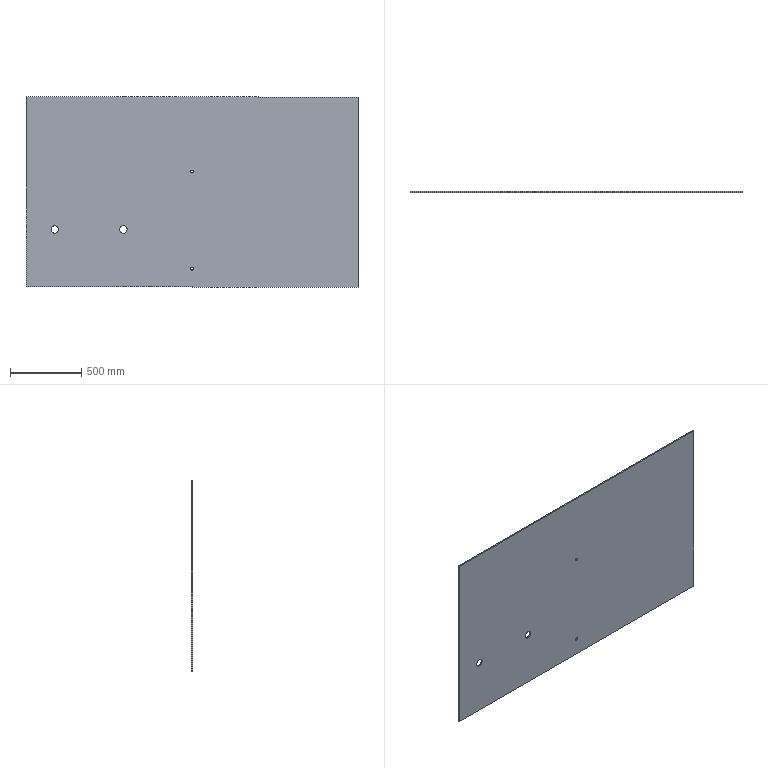Part | SolidWorks | features Extrusion 1 | 1 solid | 14 faces | box 2324 x 8 x 1330 mm | volume 24688354 mm3 | cylinder 8 | plane 6 | commonest cylinder face diameters 20 x4 52 x4
STEP:
#1=CARTESIAN_POINT('',(-960.,4.,-288.));
#2=VERTEX_POINT('',#1);
#3=CARTESIAN_POINT('',(-960.,4.,-236.));
#4=VERTEX_POINT('',#3);
#5=CARTESIAN_POINT('',(-960.,4.,-262.));
#6=DIRECTION('',(0.,1.,0.));
#7=DIRECTION('',(0.,0.,1.));
#8=AXIS2_PLACEMENT_3D('',#5,#6,#7);
#9=CIRCLE('',#8,26.);
#10=EDGE_CURVE('',#2,#4,#9,.T.);
#11=ORIENTED_EDGE('',*,*,#10,.T.);
#12=CARTESIAN_POINT('',(-960.,-4.,-236.));
#13=VERTEX_POINT('',#12);
#14=CARTESIAN_POINT('',(-960.,4.,-236.));
#15=DIRECTION('',(0.,-1.,0.));
#16=VECTOR('',#15,1000.);
#17=LINE('',#14,#16);
#18=EDGE_CURVE('',#4,#13,#17,.T.);
#19=ORIENTED_EDGE('',*,*,#18,.T.);
#20=CARTESIAN_POINT('',(-960.,-4.,-288.));
#21=VERTEX_POINT('',#20);
#22=CARTESIAN_POINT('',(-960.,-4.,-262.));
#23=DIRECTION('',(0.,1.,0.));
#24=DIRECTION('',(0.,0.,1.));
#25=AXIS2_PLACEMENT_3D('',#22,#23,#24);
#26=CIRCLE('',#25,26.);
#27=EDGE_CURVE('',#21,#13,#26,.T.);
#28=ORIENTED_EDGE('',*,*,#27,.F.);
#29=CARTESIAN_POINT('',(-960.,4.,-288.));
#30=DIRECTION('',(0.,-1.,0.));
#31=VECTOR('',#30,1000.);
#32=LINE('',#29,#31);
#33=EDGE_CURVE('',#2,#21,#32,.T.);
#34=ORIENTED_EDGE('',*,*,#33,.F.);
#35=EDGE_LOOP('',(#11,#19,#28,#34));
#36=FACE_OUTER_BOUND('',#35,.T.);
#37=CARTESIAN_POINT('',(-960.,4.,-262.));
#38=DIRECTION('',(0.,-1.,0.));
#39=DIRECTION('',(0.,0.,-1.));
#40=AXIS2_PLACEMENT_3D('',#37,#38,#39);
#41=CYLINDRICAL_SURFACE('',#40,26.);
#42=ADVANCED_FACE('',(#36),#41,.F.);
#43=CARTESIAN_POINT('',(-480.,4.,-288.));
#44=VERTEX_POINT('',#43);
#45=CARTESIAN_POINT('',(-480.,4.,-236.));
#46=VERTEX_POINT('',#45);
#47=CARTESIAN_POINT('',(-480.,4.,-262.));
#48=DIRECTION('',(0.,1.,0.));
#49=DIRECTION('',(0.,0.,1.));
#50=AXIS2_PLACEMENT_3D('',#47,#48,#49);
#51=CIRCLE('',#50,26.);
#52=EDGE_CURVE('',#44,#46,#51,.T.);
#53=ORIENTED_EDGE('',*,*,#52,.T.);
#54=CARTESIAN_POINT('',(-480.,-4.,-236.));
#55=VERTEX_POINT('',#54);
#56=CARTESIAN_POINT('',(-480.,4.,-236.));
#57=DIRECTION('',(0.,-1.,0.));
#58=VECTOR('',#57,1000.);
#59=LINE('',#56,#58);
#60=EDGE_CURVE('',#46,#55,#59,.T.);
#61=ORIENTED_EDGE('',*,*,#60,.T.);
#62=CARTESIAN_POINT('',(-480.,-4.,-288.));
#63=VERTEX_POINT('',#62);
#64=CARTESIAN_POINT('',(-480.,-4.,-262.));
#65=DIRECTION('',(0.,1.,0.));
#66=DIRECTION('',(0.,0.,1.));
#67=AXIS2_PLACEMENT_3D('',#64,#65,#66);
#68=CIRCLE('',#67,26.);
#69=EDGE_CURVE('',#63,#55,#68,.T.);
#70=ORIENTED_EDGE('',*,*,#69,.F.);
#71=CARTESIAN_POINT('',(-480.,4.,-288.));
#72=DIRECTION('',(0.,-1.,0.));
#73=VECTOR('',#72,1000.);
#74=LINE('',#71,#73);
#75=EDGE_CURVE('',#44,#63,#74,.T.);
#76=ORIENTED_EDGE('',*,*,#75,.F.);
#77=EDGE_LOOP('',(#53,#61,#70,#76));
#78=FACE_OUTER_BOUND('',#77,.T.);
#79=CARTESIAN_POINT('',(-480.,4.,-262.));
#80=DIRECTION('',(0.,-1.,0.));
#81=DIRECTION('',(0.,0.,-1.));
#82=AXIS2_PLACEMENT_3D('',#79,#80,#81);
#83=CYLINDRICAL_SURFACE('',#82,26.);
#84=ADVANCED_FACE('',(#78),#83,.F.);
#85=CARTESIAN_POINT('',(0.,4.,133.));
#86=VERTEX_POINT('',#85);
#87=CARTESIAN_POINT('',(0.,4.,153.));
#88=VERTEX_POINT('',#87);
#89=CARTESIAN_POINT('',(0.,4.,143.));
#90=DIRECTION('',(0.,1.,0.));
#91=DIRECTION('',(0.,0.,1.));
#92=AXIS2_PLACEMENT_3D('',#89,#90,#91);
#93=CIRCLE('',#92,10.);
#94=EDGE_CURVE('',#86,#88,#93,.T.);
#95=ORIENTED_EDGE('',*,*,#94,.T.);
#96=CARTESIAN_POINT('',(0.,-4.,153.));
#97=VERTEX_POINT('',#96);
#98=CARTESIAN_POINT('',(0.,4.,153.));
#99=DIRECTION('',(0.,-1.,0.));
#100=VECTOR('',#99,1000.);
#101=LINE('',#98,#100);
#102=EDGE_CURVE('',#88,#97,#101,.T.);
#103=ORIENTED_EDGE('',*,*,#102,.T.);
#104=CARTESIAN_POINT('',(0.,-4.,133.));
#105=VERTEX_POINT('',#104);
#106=CARTESIAN_POINT('',(0.,-4.,143.));
#107=DIRECTION('',(0.,1.,0.));
#108=DIRECTION('',(0.,0.,1.));
#109=AXIS2_PLACEMENT_3D('',#106,#107,#108);
#110=CIRCLE('',#109,10.);
#111=EDGE_CURVE('',#105,#97,#110,.T.);
#112=ORIENTED_EDGE('',*,*,#111,.F.);
#113=CARTESIAN_POINT('',(0.,4.,133.));
#114=DIRECTION('',(0.,-1.,0.));
#115=VECTOR('',#114,1000.);
#116=LINE('',#113,#115);
#117=EDGE_CURVE('',#86,#105,#116,.T.);
#118=ORIENTED_EDGE('',*,*,#117,.F.);
#119=EDGE_LOOP('',(#95,#103,#112,#118));
#120=FACE_OUTER_BOUND('',#119,.T.);
#121=CARTESIAN_POINT('',(0.,4.,143.));
#122=DIRECTION('',(0.,-1.,0.));
#123=DIRECTION('',(0.,0.,-1.));
#124=AXIS2_PLACEMENT_3D('',#121,#122,#123);
#125=CYLINDRICAL_SURFACE('',#124,10.);
#126=ADVANCED_FACE('',(#120),#125,.F.);
#127=CARTESIAN_POINT('',(0.,4.,-547.));
#128=VERTEX_POINT('',#127);
#129=CARTESIAN_POINT('',(0.,4.,-527.));
#130=VERTEX_POINT('',#129);
#131=CARTESIAN_POINT('',(0.,4.,-537.));
#132=DIRECTION('',(0.,1.,0.));
#133=DIRECTION('',(0.,0.,1.));
#134=AXIS2_PLACEMENT_3D('',#131,#132,#133);
#135=CIRCLE('',#134,10.);
#136=EDGE_CURVE('',#128,#130,#135,.T.);
#137=ORIENTED_EDGE('',*,*,#136,.T.);
#138=CARTESIAN_POINT('',(0.,-4.,-527.));
#139=VERTEX_POINT('',#138);
#140=CARTESIAN_POINT('',(0.,4.,-527.));
#141=DIRECTION('',(0.,-1.,0.));
#142=VECTOR('',#141,1000.);
#143=LINE('',#140,#142);
#144=EDGE_CURVE('',#130,#139,#143,.T.);
#145=ORIENTED_EDGE('',*,*,#144,.T.);
#146=CARTESIAN_POINT('',(0.,-4.,-547.));
#147=VERTEX_POINT('',#146);
#148=CARTESIAN_POINT('',(0.,-4.,-537.));
#149=DIRECTION('',(0.,1.,0.));
#150=DIRECTION('',(0.,0.,1.));
#151=AXIS2_PLACEMENT_3D('',#148,#149,#150);
#152=CIRCLE('',#151,10.);
#153=EDGE_CURVE('',#147,#139,#152,.T.);
#154=ORIENTED_EDGE('',*,*,#153,.F.);
#155=CARTESIAN_POINT('',(0.,4.,-547.));
#156=DIRECTION('',(0.,-1.,0.));
#157=VECTOR('',#156,1000.);
#158=LINE('',#155,#157);
#159=EDGE_CURVE('',#128,#147,#158,.T.);
#160=ORIENTED_EDGE('',*,*,#159,.F.);
#161=EDGE_LOOP('',(#137,#145,#154,#160));
#162=FACE_OUTER_BOUND('',#161,.T.);
#163=CARTESIAN_POINT('',(0.,4.,-537.));
#164=DIRECTION('',(0.,-1.,0.));
#165=DIRECTION('',(0.,0.,-1.));
#166=AXIS2_PLACEMENT_3D('',#163,#164,#165);
#167=CYLINDRICAL_SURFACE('',#166,10.);
#168=ADVANCED_FACE('',(#162),#167,.F.);
#169=CARTESIAN_POINT('',(1162.,4.,665.));
#170=VERTEX_POINT('',#169);
#171=CARTESIAN_POINT('',(1162.,4.,-665.));
#172=VERTEX_POINT('',#171);
#173=CARTESIAN_POINT('',(1162.,4.,665.));
#174=DIRECTION('',(0.,0.,-1.));
#175=VECTOR('',#174,1000.);
#176=LINE('',#173,#175);
#177=EDGE_CURVE('',#170,#172,#176,.T.);
#178=ORIENTED_EDGE('',*,*,#177,.T.);
#179=CARTESIAN_POINT('',(-1162.,4.,-665.));
#180=VERTEX_POINT('',#179);
#181=CARTESIAN_POINT('',(-1162.,4.,-665.));
#182=DIRECTION('',(-1.,0.,0.));
#183=VECTOR('',#182,1000.);
#184=LINE('',#181,#183);
#185=EDGE_CURVE('',#172,#180,#184,.T.);
#186=ORIENTED_EDGE('',*,*,#185,.T.);
#187=CARTESIAN_POINT('',(-1162.,4.,665.));
#188=VERTEX_POINT('',#187);
#189=CARTESIAN_POINT('',(-1162.,4.,665.));
#190=DIRECTION('',(0.,0.,1.));
#191=VECTOR('',#190,1000.);
#192=LINE('',#189,#191);
#193=EDGE_CURVE('',#180,#188,#192,.T.);
#194=ORIENTED_EDGE('',*,*,#193,.T.);
#195=CARTESIAN_POINT('',(-1162.,4.,665.));
#196=DIRECTION('',(1.,0.,0.));
#197=VECTOR('',#196,1000.);
#198=LINE('',#195,#197);
#199=EDGE_CURVE('',#188,#170,#198,.T.);
#200=ORIENTED_EDGE('',*,*,#199,.T.);
#201=EDGE_LOOP('',(#178,#186,#194,#200));
#202=FACE_OUTER_BOUND('',#201,.T.);
#203=ORIENTED_EDGE('',*,*,#136,.F.);
#204=CARTESIAN_POINT('',(0.,4.,-537.));
#205=DIRECTION('',(0.,1.,0.));
#206=DIRECTION('',(0.,0.,1.));
#207=AXIS2_PLACEMENT_3D('',#204,#205,#206);
#208=CIRCLE('',#207,10.);
#209=EDGE_CURVE('',#130,#128,#208,.T.);
#210=ORIENTED_EDGE('',*,*,#209,.F.);
#211=EDGE_LOOP('',(#203,#210));
#212=FACE_BOUND('',#211,.T.);
#213=ORIENTED_EDGE('',*,*,#94,.F.);
#214=CARTESIAN_POINT('',(0.,4.,143.));
#215=DIRECTION('',(0.,1.,0.));
#216=DIRECTION('',(0.,0.,1.));
#217=AXIS2_PLACEMENT_3D('',#214,#215,#216);
#218=CIRCLE('',#217,10.);
#219=EDGE_CURVE('',#88,#86,#218,.T.);
#220=ORIENTED_EDGE('',*,*,#219,.F.);
#221=EDGE_LOOP('',(#213,#220));
#222=FACE_BOUND('',#221,.T.);
#223=ORIENTED_EDGE('',*,*,#52,.F.);
#224=CARTESIAN_POINT('',(-480.,4.,-262.));
#225=DIRECTION('',(0.,1.,0.));
#226=DIRECTION('',(0.,0.,1.));
#227=AXIS2_PLACEMENT_3D('',#224,#225,#226);
#228=CIRCLE('',#227,26.);
#229=EDGE_CURVE('',#46,#44,#228,.T.);
#230=ORIENTED_EDGE('',*,*,#229,.F.);
#231=EDGE_LOOP('',(#223,#230));
#232=FACE_BOUND('',#231,.T.);
#233=ORIENTED_EDGE('',*,*,#10,.F.);
#234=CARTESIAN_POINT('',(-960.,4.,-262.));
#235=DIRECTION('',(0.,1.,0.));
#236=DIRECTION('',(0.,0.,1.));
#237=AXIS2_PLACEMENT_3D('',#234,#235,#236);
#238=CIRCLE('',#237,26.);
#239=EDGE_CURVE('',#4,#2,#238,.T.);
#240=ORIENTED_EDGE('',*,*,#239,.F.);
#241=EDGE_LOOP('',(#233,#240));
#242=FACE_BOUND('',#241,.T.);
#243=CARTESIAN_POINT('',(0.,4.,0.));
#244=DIRECTION('',(0.,-1.,0.));
#245=DIRECTION('',(0.,0.,-1.));
#246=AXIS2_PLACEMENT_3D('',#243,#244,#245);
#247=PLANE('',#246);
#248=ADVANCED_FACE('',(#202,#212,#222,#232,#242),#247,.F.);
#249=ORIENTED_EDGE('',*,*,#69,.T.);
#250=CARTESIAN_POINT('',(-480.,-4.,-262.));
#251=DIRECTION('',(0.,1.,0.));
#252=DIRECTION('',(0.,0.,1.));
#253=AXIS2_PLACEMENT_3D('',#250,#251,#252);
#254=CIRCLE('',#253,26.);
#255=EDGE_CURVE('',#55,#63,#254,.T.);
#256=ORIENTED_EDGE('',*,*,#255,.T.);
#257=EDGE_LOOP('',(#249,#256));
#258=FACE_BOUND('',#257,.T.);
#259=ORIENTED_EDGE('',*,*,#153,.T.);
#260=CARTESIAN_POINT('',(0.,-4.,-537.));
#261=DIRECTION('',(0.,1.,0.));
#262=DIRECTION('',(0.,0.,1.));
#263=AXIS2_PLACEMENT_3D('',#260,#261,#262);
#264=CIRCLE('',#263,10.);
#265=EDGE_CURVE('',#139,#147,#264,.T.);
#266=ORIENTED_EDGE('',*,*,#265,.T.);
#267=EDGE_LOOP('',(#259,#266));
#268=FACE_BOUND('',#267,.T.);
#269=CARTESIAN_POINT('',(1162.,-4.,665.));
#270=VERTEX_POINT('',#269);
#271=CARTESIAN_POINT('',(1162.,-4.,-665.));
#272=VERTEX_POINT('',#271);
#273=CARTESIAN_POINT('',(1162.,-4.,665.));
#274=DIRECTION('',(0.,0.,-1.));
#275=VECTOR('',#274,1000.);
#276=LINE('',#273,#275);
#277=EDGE_CURVE('',#270,#272,#276,.T.);
#278=ORIENTED_EDGE('',*,*,#277,.F.);
#279=CARTESIAN_POINT('',(-1162.,-4.,665.));
#280=VERTEX_POINT('',#279);
#281=CARTESIAN_POINT('',(-1162.,-4.,665.));
#282=DIRECTION('',(1.,0.,0.));
#283=VECTOR('',#282,1000.);
#284=LINE('',#281,#283);
#285=EDGE_CURVE('',#280,#270,#284,.T.);
#286=ORIENTED_EDGE('',*,*,#285,.F.);
#287=CARTESIAN_POINT('',(-1162.,-4.,-665.));
#288=VERTEX_POINT('',#287);
#289=CARTESIAN_POINT('',(-1162.,-4.,665.));
#290=DIRECTION('',(0.,0.,1.));
#291=VECTOR('',#290,1000.);
#292=LINE('',#289,#291);
#293=EDGE_CURVE('',#288,#280,#292,.T.);
#294=ORIENTED_EDGE('',*,*,#293,.F.);
#295=CARTESIAN_POINT('',(-1162.,-4.,-665.));
#296=DIRECTION('',(-1.,0.,0.));
#297=VECTOR('',#296,1000.);
#298=LINE('',#295,#297);
#299=EDGE_CURVE('',#272,#288,#298,.T.);
#300=ORIENTED_EDGE('',*,*,#299,.F.);
#301=EDGE_LOOP('',(#278,#286,#294,#300));
#302=FACE_OUTER_BOUND('',#301,.T.);
#303=ORIENTED_EDGE('',*,*,#111,.T.);
#304=CARTESIAN_POINT('',(0.,-4.,143.));
#305=DIRECTION('',(0.,1.,0.));
#306=DIRECTION('',(0.,0.,1.));
#307=AXIS2_PLACEMENT_3D('',#304,#305,#306);
#308=CIRCLE('',#307,10.);
#309=EDGE_CURVE('',#97,#105,#308,.T.);
#310=ORIENTED_EDGE('',*,*,#309,.T.);
#311=EDGE_LOOP('',(#303,#310));
#312=FACE_BOUND('',#311,.T.);
#313=ORIENTED_EDGE('',*,*,#27,.T.);
#314=CARTESIAN_POINT('',(-960.,-4.,-262.));
#315=DIRECTION('',(0.,1.,0.));
#316=DIRECTION('',(0.,0.,1.));
#317=AXIS2_PLACEMENT_3D('',#314,#315,#316);
#318=CIRCLE('',#317,26.);
#319=EDGE_CURVE('',#13,#21,#318,.T.);
#320=ORIENTED_EDGE('',*,*,#319,.T.);
#321=EDGE_LOOP('',(#313,#320));
#322=FACE_BOUND('',#321,.T.);
#323=CARTESIAN_POINT('',(0.,-4.,0.));
#324=DIRECTION('',(0.,-1.,0.));
#325=DIRECTION('',(0.,0.,-1.));
#326=AXIS2_PLACEMENT_3D('',#323,#324,#325);
#327=PLANE('',#326);
#328=ADVANCED_FACE('',(#258,#268,#302,#312,#322),#327,.T.);
#329=ORIENTED_EDGE('',*,*,#277,.T.);
#330=CARTESIAN_POINT('',(1162.,4.,-665.));
#331=DIRECTION('',(0.,-1.,0.));
#332=VECTOR('',#331,1000.);
#333=LINE('',#330,#332);
#334=EDGE_CURVE('',#172,#272,#333,.T.);
#335=ORIENTED_EDGE('',*,*,#334,.F.);
#336=ORIENTED_EDGE('',*,*,#177,.F.);
#337=CARTESIAN_POINT('',(1162.,4.,665.));
#338=DIRECTION('',(0.,-1.,0.));
#339=VECTOR('',#338,1000.);
#340=LINE('',#337,#339);
#341=EDGE_CURVE('',#170,#270,#340,.T.);
#342=ORIENTED_EDGE('',*,*,#341,.T.);
#343=EDGE_LOOP('',(#329,#335,#336,#342));
#344=FACE_OUTER_BOUND('',#343,.T.);
#345=CARTESIAN_POINT('',(1162.,4.,665.));
#346=DIRECTION('',(-1.,0.,0.));
#347=DIRECTION('',(0.,0.,1.));
#348=AXIS2_PLACEMENT_3D('',#345,#346,#347);
#349=PLANE('',#348);
#350=ADVANCED_FACE('',(#344),#349,.F.);
#351=ORIENTED_EDGE('',*,*,#299,.T.);
#352=CARTESIAN_POINT('',(-1162.,4.,-665.));
#353=DIRECTION('',(0.,-1.,0.));
#354=VECTOR('',#353,1000.);
#355=LINE('',#352,#354);
#356=EDGE_CURVE('',#180,#288,#355,.T.);
#357=ORIENTED_EDGE('',*,*,#356,.F.);
#358=ORIENTED_EDGE('',*,*,#185,.F.);
#359=ORIENTED_EDGE('',*,*,#334,.T.);
#360=EDGE_LOOP('',(#351,#357,#358,#359));
#361=FACE_OUTER_BOUND('',#360,.T.);
#362=CARTESIAN_POINT('',(-1162.,4.,-665.));
#363=DIRECTION('',(0.,0.,1.));
#364=DIRECTION('',(1.,0.,0.));
#365=AXIS2_PLACEMENT_3D('',#362,#363,#364);
#366=PLANE('',#365);
#367=ADVANCED_FACE('',(#361),#366,.F.);
#368=ORIENTED_EDGE('',*,*,#293,.T.);
#369=CARTESIAN_POINT('',(-1162.,4.,665.));
#370=DIRECTION('',(0.,-1.,0.));
#371=VECTOR('',#370,1000.);
#372=LINE('',#369,#371);
#373=EDGE_CURVE('',#188,#280,#372,.T.);
#374=ORIENTED_EDGE('',*,*,#373,.F.);
#375=ORIENTED_EDGE('',*,*,#193,.F.);
#376=ORIENTED_EDGE('',*,*,#356,.T.);
#377=EDGE_LOOP('',(#368,#374,#375,#376));
#378=FACE_OUTER_BOUND('',#377,.T.);
#379=CARTESIAN_POINT('',(-1162.,4.,665.));
#380=DIRECTION('',(1.,0.,0.));
#381=DIRECTION('',(0.,0.,-1.));
#382=AXIS2_PLACEMENT_3D('',#379,#380,#381);
#383=PLANE('',#382);
#384=ADVANCED_FACE('',(#378),#383,.F.);
#385=ORIENTED_EDGE('',*,*,#285,.T.);
#386=ORIENTED_EDGE('',*,*,#341,.F.);
#387=ORIENTED_EDGE('',*,*,#199,.F.);
#388=ORIENTED_EDGE('',*,*,#373,.T.);
#389=EDGE_LOOP('',(#385,#386,#387,#388));
#390=FACE_OUTER_BOUND('',#389,.T.);
#391=CARTESIAN_POINT('',(-1162.,4.,665.));
#392=DIRECTION('',(0.,0.,-1.));
#393=DIRECTION('',(-1.,0.,0.));
#394=AXIS2_PLACEMENT_3D('',#391,#392,#393);
#395=PLANE('',#394);
#396=ADVANCED_FACE('',(#390),#395,.F.);
#397=ORIENTED_EDGE('',*,*,#144,.F.);
#398=ORIENTED_EDGE('',*,*,#209,.T.);
#399=ORIENTED_EDGE('',*,*,#159,.T.);
#400=ORIENTED_EDGE('',*,*,#265,.F.);
#401=EDGE_LOOP('',(#397,#398,#399,#400));
#402=FACE_OUTER_BOUND('',#401,.T.);
#403=CARTESIAN_POINT('',(0.,4.,-537.));
#404=DIRECTION('',(0.,-1.,0.));
#405=DIRECTION('',(0.,0.,-1.));
#406=AXIS2_PLACEMENT_3D('',#403,#404,#405);
#407=CYLINDRICAL_SURFACE('',#406,10.);
#408=ADVANCED_FACE('',(#402),#407,.F.);
#409=ORIENTED_EDGE('',*,*,#102,.F.);
#410=ORIENTED_EDGE('',*,*,#219,.T.);
#411=ORIENTED_EDGE('',*,*,#117,.T.);
#412=ORIENTED_EDGE('',*,*,#309,.F.);
#413=EDGE_LOOP('',(#409,#410,#411,#412));
#414=FACE_OUTER_BOUND('',#413,.T.);
#415=CARTESIAN_POINT('',(0.,4.,143.));
#416=DIRECTION('',(0.,-1.,0.));
#417=DIRECTION('',(0.,0.,-1.));
#418=AXIS2_PLACEMENT_3D('',#415,#416,#417);
#419=CYLINDRICAL_SURFACE('',#418,10.);
#420=ADVANCED_FACE('',(#414),#419,.F.);
#421=ORIENTED_EDGE('',*,*,#60,.F.);
#422=ORIENTED_EDGE('',*,*,#229,.T.);
#423=ORIENTED_EDGE('',*,*,#75,.T.);
#424=ORIENTED_EDGE('',*,*,#255,.F.);
#425=EDGE_LOOP('',(#421,#422,#423,#424));
#426=FACE_OUTER_BOUND('',#425,.T.);
#427=CARTESIAN_POINT('',(-480.,4.,-262.));
#428=DIRECTION('',(0.,-1.,0.));
#429=DIRECTION('',(0.,0.,-1.));
#430=AXIS2_PLACEMENT_3D('',#427,#428,#429);
#431=CYLINDRICAL_SURFACE('',#430,26.);
#432=ADVANCED_FACE('',(#426),#431,.F.);
#433=ORIENTED_EDGE('',*,*,#18,.F.);
#434=ORIENTED_EDGE('',*,*,#239,.T.);
#435=ORIENTED_EDGE('',*,*,#33,.T.);
#436=ORIENTED_EDGE('',*,*,#319,.F.);
#437=EDGE_LOOP('',(#433,#434,#435,#436));
#438=FACE_OUTER_BOUND('',#437,.T.);
#439=CARTESIAN_POINT('',(-960.,4.,-262.));
#440=DIRECTION('',(0.,-1.,0.));
#441=DIRECTION('',(0.,0.,-1.));
#442=AXIS2_PLACEMENT_3D('',#439,#440,#441);
#443=CYLINDRICAL_SURFACE('',#442,26.);
#444=ADVANCED_FACE('',(#438),#443,.F.);
#445=CLOSED_SHELL('',(#42,#84,#126,#168,#248,#328,#350,#367,#384,#396,#408,#420,#432,#444));
#446=MANIFOLD_SOLID_BREP('',#445);
#447=CARTESIAN_POINT('',(0.,0.,0.));
#448=DIRECTION('',(0.,0.,1.));
#449=DIRECTION('',(1.,0.,0.));
#450=AXIS2_PLACEMENT_3D('',#447,#448,#449);
#451=(LENGTH_UNIT()NAMED_UNIT(*)SI_UNIT(.MILLI.,.METRE.));
#452=UNCERTAINTY_MEASURE_WITH_UNIT(LENGTH_MEASURE(0.00001),#451,'','');
#453=(NAMED_UNIT(*)PLANE_ANGLE_UNIT()SI_UNIT($,.RADIAN.));
#454=(NAMED_UNIT(*)SI_UNIT($,.STERADIAN.)SOLID_ANGLE_UNIT());
#455=(GEOMETRIC_REPRESENTATION_CONTEXT(3)GLOBAL_UNCERTAINTY_ASSIGNED_CONTEXT((#452))GLOBAL_UNIT_ASSIGNED_CONTEXT((#451,#453,#454))REPRESENTATION_CONTEXT('',''));
#456=ADVANCED_BREP_SHAPE_REPRESENTATION('',(#446,#450),#455);